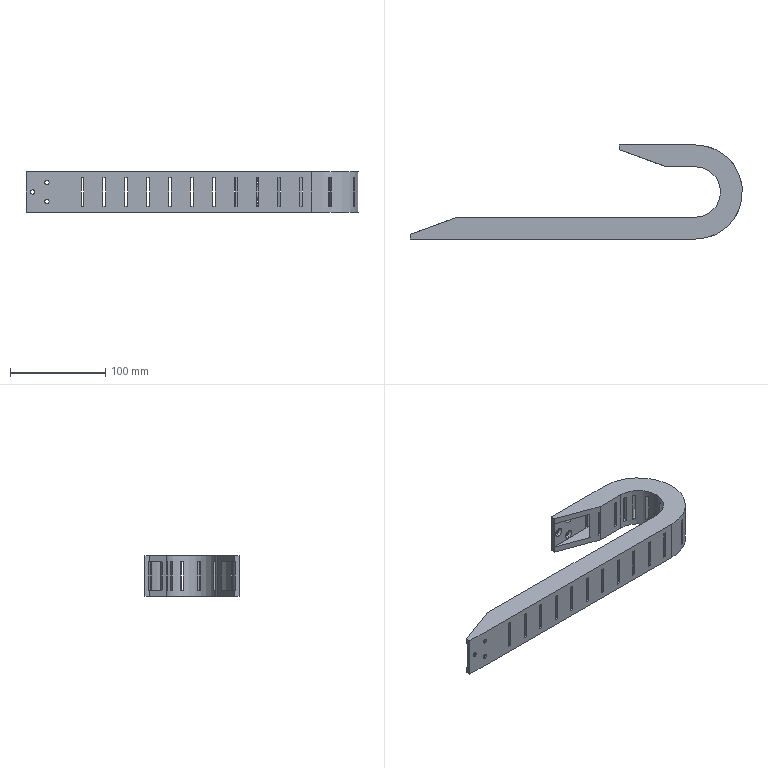Part | STEP file | TP15.30(Ruiao) | 1 solid | 154 faces | box 349.5 x 99 x 43 mm | volume 233329 mm3 | plane 114 | cylinder 28 | cone 12 | commonest cylinder face diameters 4.5 x12 61 x7 91 x7 53 x1 99 x1